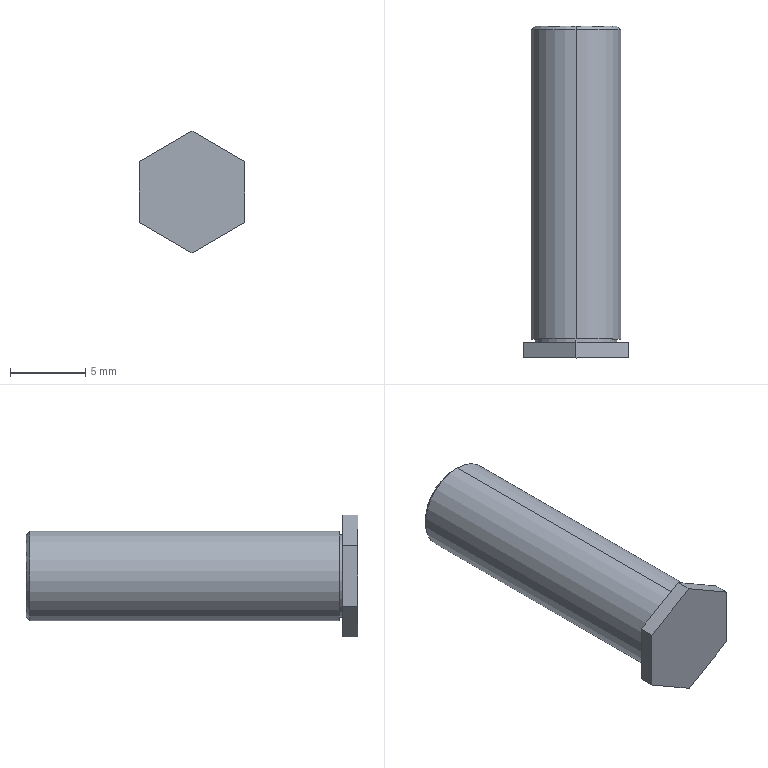Part | NX | features BREP 1 | 1 solid | 21 faces | box 7 x 22 x 8.083 mm | volume 461.807 mm3 | plane 11 | cylinder 6 | cone 4 | commonest cylinder face diameters 3.3 x2 5.45 x2 5.95 x2
STEP:
#1=CARTESIAN_POINT('',(300.5,43.15,424.025));
#2=VERTEX_POINT('',#1);
#3=CARTESIAN_POINT('',(300.5,43.15,429.975));
#4=VERTEX_POINT('',#3);
#5=CARTESIAN_POINT('',(300.5,43.15,427.));
#6=DIRECTION('',(0.,-1.,0.));
#7=DIRECTION('',(0.,0.,-1.));
#8=AXIS2_PLACEMENT_3D('',#5,#6,#7);
#9=CIRCLE('',#8,2.975);
#10=EDGE_CURVE('',#2,#4,#9,.T.);
#11=ORIENTED_EDGE('',*,*,#10,.T.);
#12=CARTESIAN_POINT('',(300.5,22.65,429.975));
#13=VERTEX_POINT('',#12);
#14=CARTESIAN_POINT('',(300.5,31.4,429.975));
#15=DIRECTION('',(0.,-1.,0.));
#16=VECTOR('',#15,1000.);
#17=LINE('',#14,#16);
#18=EDGE_CURVE('',#13,#4,#17,.F.);
#19=ORIENTED_EDGE('',*,*,#18,.F.);
#20=CARTESIAN_POINT('',(300.5,22.65,424.025));
#21=VERTEX_POINT('',#20);
#22=CARTESIAN_POINT('',(300.5,22.65,427.));
#23=DIRECTION('',(0.,1.,0.));
#24=DIRECTION('',(0.,0.,-1.));
#25=AXIS2_PLACEMENT_3D('',#22,#23,#24);
#26=CIRCLE('',#25,2.975);
#27=EDGE_CURVE('',#13,#21,#26,.T.);
#28=ORIENTED_EDGE('',*,*,#27,.T.);
#29=CARTESIAN_POINT('',(300.5,31.4,424.025));
#30=DIRECTION('',(0.,-1.,0.));
#31=VECTOR('',#30,1000.);
#32=LINE('',#29,#31);
#33=EDGE_CURVE('',#21,#2,#32,.F.);
#34=ORIENTED_EDGE('',*,*,#33,.T.);
#35=EDGE_LOOP('',(#11,#19,#28,#34));
#36=FACE_BOUND('',#35,.T.);
#37=CARTESIAN_POINT('',(300.5,31.4,427.));
#38=DIRECTION('',(0.,-1.,0.));
#39=DIRECTION('',(0.,0.,1.));
#40=AXIS2_PLACEMENT_3D('',#37,#38,#39);
#41=CYLINDRICAL_SURFACE('',#40,2.975);
#42=ADVANCED_FACE('',(#36),#41,.T.);
#43=CARTESIAN_POINT('',(300.5,43.4,424.275));
#44=VERTEX_POINT('',#43);
#45=CARTESIAN_POINT('',(300.5,43.4,429.725));
#46=VERTEX_POINT('',#45);
#47=CARTESIAN_POINT('',(300.5,43.4,427.));
#48=DIRECTION('',(0.,-1.,0.));
#49=DIRECTION('',(0.,0.,-1.));
#50=AXIS2_PLACEMENT_3D('',#47,#48,#49);
#51=CIRCLE('',#50,2.725);
#52=EDGE_CURVE('',#44,#46,#51,.T.);
#53=ORIENTED_EDGE('',*,*,#52,.T.);
#54=CARTESIAN_POINT('',(300.5,43.15,429.975));
#55=DIRECTION('',(0.,-0.7071,0.7071));
#56=VECTOR('',#55,1000.);
#57=LINE('',#54,#56);
#58=EDGE_CURVE('',#4,#46,#57,.F.);
#59=ORIENTED_EDGE('',*,*,#58,.F.);
#60=ORIENTED_EDGE('',*,*,#10,.F.);
#61=CARTESIAN_POINT('',(300.5,43.15,424.025));
#62=DIRECTION('',(0.,-0.7071,-0.7071));
#63=VECTOR('',#62,1000.);
#64=LINE('',#61,#63);
#65=EDGE_CURVE('',#2,#44,#64,.F.);
#66=ORIENTED_EDGE('',*,*,#65,.T.);
#67=EDGE_LOOP('',(#53,#59,#60,#66));
#68=FACE_BOUND('',#67,.T.);
#69=CARTESIAN_POINT('',(300.5,43.15,427.));
#70=DIRECTION('',(0.,-1.,0.));
#71=DIRECTION('',(0.,0.,1.));
#72=AXIS2_PLACEMENT_3D('',#69,#70,#71);
#73=CONICAL_SURFACE('',#72,2.975,0.7854);
#74=ADVANCED_FACE('',(#68),#73,.T.);
#75=CARTESIAN_POINT('',(300.5,22.4,429.725));
#76=VERTEX_POINT('',#75);
#77=CARTESIAN_POINT('',(300.5,22.4,424.275));
#78=VERTEX_POINT('',#77);
#79=CARTESIAN_POINT('',(300.5,22.4,427.));
#80=DIRECTION('',(0.,1.,0.));
#81=DIRECTION('',(0.,0.,1.));
#82=AXIS2_PLACEMENT_3D('',#79,#80,#81);
#83=CIRCLE('',#82,2.725);
#84=EDGE_CURVE('',#76,#78,#83,.T.);
#85=ORIENTED_EDGE('',*,*,#84,.T.);
#86=CARTESIAN_POINT('',(300.5,22.65,424.275));
#87=VERTEX_POINT('',#86);
#88=CARTESIAN_POINT('',(300.5,-1.133,424.275));
#89=DIRECTION('',(0.,1.,0.));
#90=VECTOR('',#89,1000.);
#91=LINE('',#88,#90);
#92=EDGE_CURVE('',#78,#87,#91,.T.);
#93=ORIENTED_EDGE('',*,*,#92,.T.);
#94=CARTESIAN_POINT('',(300.5,22.65,429.725));
#95=VERTEX_POINT('',#94);
#96=CARTESIAN_POINT('',(300.5,22.65,427.));
#97=DIRECTION('',(0.,-1.,0.));
#98=DIRECTION('',(0.,0.,1.));
#99=AXIS2_PLACEMENT_3D('',#96,#97,#98);
#100=CIRCLE('',#99,2.725);
#101=EDGE_CURVE('',#87,#95,#100,.T.);
#102=ORIENTED_EDGE('',*,*,#101,.T.);
#103=CARTESIAN_POINT('',(300.5,-1.133,429.725));
#104=DIRECTION('',(0.,1.,0.));
#105=VECTOR('',#104,1000.);
#106=LINE('',#103,#105);
#107=EDGE_CURVE('',#76,#95,#106,.T.);
#108=ORIENTED_EDGE('',*,*,#107,.F.);
#109=EDGE_LOOP('',(#85,#93,#102,#108));
#110=FACE_BOUND('',#109,.T.);
#111=CARTESIAN_POINT('',(300.5,-1.133,427.));
#112=DIRECTION('',(0.,1.,0.));
#113=DIRECTION('',(0.,0.,-1.));
#114=AXIS2_PLACEMENT_3D('',#111,#112,#113);
#115=CYLINDRICAL_SURFACE('',#114,2.725);
#116=ADVANCED_FACE('',(#110),#115,.T.);
#117=CARTESIAN_POINT('',(300.5,43.15,425.35));
#118=VERTEX_POINT('',#117);
#119=CARTESIAN_POINT('',(300.5,43.15,428.65));
#120=VERTEX_POINT('',#119);
#121=CARTESIAN_POINT('',(300.5,43.15,427.));
#122=DIRECTION('',(0.,1.,0.));
#123=DIRECTION('',(0.,0.,1.));
#124=AXIS2_PLACEMENT_3D('',#121,#122,#123);
#125=CIRCLE('',#124,1.65);
#126=EDGE_CURVE('',#118,#120,#125,.T.);
#127=ORIENTED_EDGE('',*,*,#126,.F.);
#128=CARTESIAN_POINT('',(300.5,43.4,425.1));
#129=VERTEX_POINT('',#128);
#130=CARTESIAN_POINT('',(300.5,43.4,425.1));
#131=DIRECTION('',(0.,0.7071,-0.7071));
#132=VECTOR('',#131,1000.);
#133=LINE('',#130,#132);
#134=EDGE_CURVE('',#118,#129,#133,.T.);
#135=ORIENTED_EDGE('',*,*,#134,.T.);
#136=CARTESIAN_POINT('',(300.5,43.4,428.9));
#137=VERTEX_POINT('',#136);
#138=CARTESIAN_POINT('',(300.5,43.4,427.));
#139=DIRECTION('',(0.,-1.,0.));
#140=DIRECTION('',(0.,0.,1.));
#141=AXIS2_PLACEMENT_3D('',#138,#139,#140);
#142=CIRCLE('',#141,1.9);
#143=EDGE_CURVE('',#137,#129,#142,.T.);
#144=ORIENTED_EDGE('',*,*,#143,.F.);
#145=CARTESIAN_POINT('',(300.5,43.4,428.9));
#146=DIRECTION('',(0.,0.7071,0.7071));
#147=VECTOR('',#146,1000.);
#148=LINE('',#145,#147);
#149=EDGE_CURVE('',#120,#137,#148,.T.);
#150=ORIENTED_EDGE('',*,*,#149,.F.);
#151=EDGE_LOOP('',(#127,#135,#144,#150));
#152=FACE_BOUND('',#151,.T.);
#153=CARTESIAN_POINT('',(300.5,43.4,427.));
#154=DIRECTION('',(0.,1.,0.));
#155=DIRECTION('',(0.,0.,-1.));
#156=AXIS2_PLACEMENT_3D('',#153,#154,#155);
#157=CONICAL_SURFACE('',#156,1.9,0.7854);
#158=ADVANCED_FACE('',(#152),#157,.F.);
#159=CARTESIAN_POINT('',(300.5,24.4,425.35));
#160=VERTEX_POINT('',#159);
#161=CARTESIAN_POINT('',(300.5,24.4,428.65));
#162=VERTEX_POINT('',#161);
#163=CARTESIAN_POINT('',(300.5,24.4,427.));
#164=DIRECTION('',(0.,1.,0.));
#165=DIRECTION('',(0.,0.,1.));
#166=AXIS2_PLACEMENT_3D('',#163,#164,#165);
#167=CIRCLE('',#166,1.65);
#168=EDGE_CURVE('',#160,#162,#167,.T.);
#169=ORIENTED_EDGE('',*,*,#168,.F.);
#170=CARTESIAN_POINT('',(300.5,24.4,425.35));
#171=DIRECTION('',(0.,1.,0.));
#172=VECTOR('',#171,1000.);
#173=LINE('',#170,#172);
#174=EDGE_CURVE('',#160,#118,#173,.T.);
#175=ORIENTED_EDGE('',*,*,#174,.T.);
#176=ORIENTED_EDGE('',*,*,#126,.T.);
#177=CARTESIAN_POINT('',(300.5,24.4,428.65));
#178=DIRECTION('',(0.,1.,0.));
#179=VECTOR('',#178,1000.);
#180=LINE('',#177,#179);
#181=EDGE_CURVE('',#162,#120,#180,.T.);
#182=ORIENTED_EDGE('',*,*,#181,.F.);
#183=EDGE_LOOP('',(#169,#175,#176,#182));
#184=FACE_BOUND('',#183,.T.);
#185=CARTESIAN_POINT('',(300.5,24.4,427.));
#186=DIRECTION('',(0.,1.,0.));
#187=DIRECTION('',(0.,0.,-1.));
#188=AXIS2_PLACEMENT_3D('',#185,#186,#187);
#189=CYLINDRICAL_SURFACE('',#188,1.65);
#190=ADVANCED_FACE('',(#184),#189,.F.);
#191=ORIENTED_EDGE('',*,*,#18,.T.);
#192=CARTESIAN_POINT('',(300.5,43.15,427.));
#193=DIRECTION('',(0.,-1.,0.));
#194=DIRECTION('',(0.,0.,-1.));
#195=AXIS2_PLACEMENT_3D('',#192,#193,#194);
#196=CIRCLE('',#195,2.975);
#197=EDGE_CURVE('',#4,#2,#196,.T.);
#198=ORIENTED_EDGE('',*,*,#197,.T.);
#199=ORIENTED_EDGE('',*,*,#33,.F.);
#200=CARTESIAN_POINT('',(300.5,22.65,427.));
#201=DIRECTION('',(0.,1.,0.));
#202=DIRECTION('',(0.,0.,-1.));
#203=AXIS2_PLACEMENT_3D('',#200,#201,#202);
#204=CIRCLE('',#203,2.975);
#205=EDGE_CURVE('',#21,#13,#204,.T.);
#206=ORIENTED_EDGE('',*,*,#205,.T.);
#207=EDGE_LOOP('',(#191,#198,#199,#206));
#208=FACE_BOUND('',#207,.T.);
#209=CARTESIAN_POINT('',(300.5,31.4,427.));
#210=DIRECTION('',(0.,-1.,0.));
#211=DIRECTION('',(0.,0.,1.));
#212=AXIS2_PLACEMENT_3D('',#209,#210,#211);
#213=CYLINDRICAL_SURFACE('',#212,2.975);
#214=ADVANCED_FACE('',(#208),#213,.T.);
#215=ORIENTED_EDGE('',*,*,#205,.F.);
#216=ORIENTED_EDGE('',*,*,#27,.F.);
#217=EDGE_LOOP('',(#215,#216));
#218=FACE_BOUND('',#217,.T.);
#219=CARTESIAN_POINT('',(300.5,22.65,427.));
#220=DIRECTION('',(0.,-1.,0.));
#221=DIRECTION('',(0.,0.,1.));
#222=AXIS2_PLACEMENT_3D('',#219,#220,#221);
#223=CIRCLE('',#222,2.725);
#224=EDGE_CURVE('',#95,#87,#223,.T.);
#225=ORIENTED_EDGE('',*,*,#224,.F.);
#226=ORIENTED_EDGE('',*,*,#101,.F.);
#227=EDGE_LOOP('',(#225,#226));
#228=FACE_BOUND('',#227,.T.);
#229=CARTESIAN_POINT('',(300.5,22.65,427.));
#230=DIRECTION('',(0.,1.,0.));
#231=DIRECTION('',(0.,0.,-1.));
#232=AXIS2_PLACEMENT_3D('',#229,#230,#231);
#233=PLANE('',#232);
#234=ADVANCED_FACE('',(#218,#228),#233,.F.);
#235=ORIENTED_EDGE('',*,*,#58,.T.);
#236=CARTESIAN_POINT('',(300.5,43.4,427.));
#237=DIRECTION('',(0.,-1.,0.));
#238=DIRECTION('',(0.,0.,-1.));
#239=AXIS2_PLACEMENT_3D('',#236,#237,#238);
#240=CIRCLE('',#239,2.725);
#241=EDGE_CURVE('',#46,#44,#240,.T.);
#242=ORIENTED_EDGE('',*,*,#241,.T.);
#243=ORIENTED_EDGE('',*,*,#65,.F.);
#244=ORIENTED_EDGE('',*,*,#197,.F.);
#245=EDGE_LOOP('',(#235,#242,#243,#244));
#246=FACE_BOUND('',#245,.T.);
#247=CARTESIAN_POINT('',(300.5,43.15,427.));
#248=DIRECTION('',(0.,-1.,0.));
#249=DIRECTION('',(0.,0.,1.));
#250=AXIS2_PLACEMENT_3D('',#247,#248,#249);
#251=CONICAL_SURFACE('',#250,2.975,0.7854);
#252=ADVANCED_FACE('',(#246),#251,.T.);
#253=ORIENTED_EDGE('',*,*,#92,.F.);
#254=CARTESIAN_POINT('',(300.5,22.4,427.));
#255=DIRECTION('',(0.,1.,0.));
#256=DIRECTION('',(0.,0.,1.));
#257=AXIS2_PLACEMENT_3D('',#254,#255,#256);
#258=CIRCLE('',#257,2.725);
#259=EDGE_CURVE('',#78,#76,#258,.T.);
#260=ORIENTED_EDGE('',*,*,#259,.T.);
#261=ORIENTED_EDGE('',*,*,#107,.T.);
#262=ORIENTED_EDGE('',*,*,#224,.T.);
#263=EDGE_LOOP('',(#253,#260,#261,#262));
#264=FACE_BOUND('',#263,.T.);
#265=CARTESIAN_POINT('',(300.5,-1.133,427.));
#266=DIRECTION('',(0.,1.,0.));
#267=DIRECTION('',(0.,0.,-1.));
#268=AXIS2_PLACEMENT_3D('',#265,#266,#267);
#269=CYLINDRICAL_SURFACE('',#268,2.725);
#270=ADVANCED_FACE('',(#264),#269,.T.);
#271=ORIENTED_EDGE('',*,*,#52,.F.);
#272=ORIENTED_EDGE('',*,*,#241,.F.);
#273=EDGE_LOOP('',(#271,#272));
#274=FACE_BOUND('',#273,.T.);
#275=ORIENTED_EDGE('',*,*,#143,.T.);
#276=CARTESIAN_POINT('',(300.5,43.4,427.));
#277=DIRECTION('',(0.,-1.,0.));
#278=DIRECTION('',(0.,0.,1.));
#279=AXIS2_PLACEMENT_3D('',#276,#277,#278);
#280=CIRCLE('',#279,1.9);
#281=EDGE_CURVE('',#129,#137,#280,.T.);
#282=ORIENTED_EDGE('',*,*,#281,.T.);
#283=EDGE_LOOP('',(#275,#282));
#284=FACE_BOUND('',#283,.T.);
#285=CARTESIAN_POINT('',(300.5,43.4,427.));
#286=DIRECTION('',(0.,1.,0.));
#287=DIRECTION('',(0.,0.,-1.));
#288=AXIS2_PLACEMENT_3D('',#285,#286,#287);
#289=PLANE('',#288);
#290=ADVANCED_FACE('',(#274,#284),#289,.T.);
#291=CARTESIAN_POINT('',(300.5,22.4,422.959));
#292=VERTEX_POINT('',#291);
#293=CARTESIAN_POINT('',(297.,22.4,424.979));
#294=VERTEX_POINT('',#293);
#295=CARTESIAN_POINT('',(300.5,22.4,422.959));
#296=DIRECTION('',(-0.866,0.,0.5));
#297=VECTOR('',#296,1000.);
#298=LINE('',#295,#297);
#299=EDGE_CURVE('',#292,#294,#298,.T.);
#300=ORIENTED_EDGE('',*,*,#299,.T.);
#301=CARTESIAN_POINT('',(297.,22.4,429.021));
#302=VERTEX_POINT('',#301);
#303=CARTESIAN_POINT('',(297.,22.4,427.));
#304=DIRECTION('',(0.,0.,1.));
#305=VECTOR('',#304,1000.);
#306=LINE('',#303,#305);
#307=EDGE_CURVE('',#294,#302,#306,.T.);
#308=ORIENTED_EDGE('',*,*,#307,.T.);
#309=CARTESIAN_POINT('',(300.5,22.4,431.041));
#310=VERTEX_POINT('',#309);
#311=CARTESIAN_POINT('',(297.,22.4,429.021));
#312=DIRECTION('',(0.866,0.,0.5));
#313=VECTOR('',#312,1000.);
#314=LINE('',#311,#313);
#315=EDGE_CURVE('',#302,#310,#314,.T.);
#316=ORIENTED_EDGE('',*,*,#315,.T.);
#317=CARTESIAN_POINT('',(304.,22.4,429.021));
#318=VERTEX_POINT('',#317);
#319=CARTESIAN_POINT('',(300.5,22.4,431.041));
#320=DIRECTION('',(0.866,0.,-0.5));
#321=VECTOR('',#320,1000.);
#322=LINE('',#319,#321);
#323=EDGE_CURVE('',#310,#318,#322,.T.);
#324=ORIENTED_EDGE('',*,*,#323,.T.);
#325=CARTESIAN_POINT('',(304.,22.4,424.979));
#326=VERTEX_POINT('',#325);
#327=CARTESIAN_POINT('',(304.,22.4,427.));
#328=DIRECTION('',(0.,0.,-1.));
#329=VECTOR('',#328,1000.);
#330=LINE('',#327,#329);
#331=EDGE_CURVE('',#318,#326,#330,.T.);
#332=ORIENTED_EDGE('',*,*,#331,.T.);
#333=CARTESIAN_POINT('',(304.,22.4,424.979));
#334=DIRECTION('',(-0.866,0.,-0.5));
#335=VECTOR('',#334,1000.);
#336=LINE('',#333,#335);
#337=EDGE_CURVE('',#326,#292,#336,.T.);
#338=ORIENTED_EDGE('',*,*,#337,.T.);
#339=EDGE_LOOP('',(#300,#308,#316,#324,#332,#338));
#340=FACE_BOUND('',#339,.T.);
#341=ORIENTED_EDGE('',*,*,#84,.F.);
#342=ORIENTED_EDGE('',*,*,#259,.F.);
#343=EDGE_LOOP('',(#341,#342));
#344=FACE_BOUND('',#343,.T.);
#345=CARTESIAN_POINT('',(300.5,22.4,427.));
#346=DIRECTION('',(0.,1.,0.));
#347=DIRECTION('',(0.,0.,-1.));
#348=AXIS2_PLACEMENT_3D('',#345,#346,#347);
#349=PLANE('',#348);
#350=ADVANCED_FACE('',(#340,#344),#349,.T.);
#351=ORIENTED_EDGE('',*,*,#134,.F.);
#352=CARTESIAN_POINT('',(300.5,43.15,427.));
#353=DIRECTION('',(0.,1.,0.));
#354=DIRECTION('',(0.,0.,1.));
#355=AXIS2_PLACEMENT_3D('',#352,#353,#354);
#356=CIRCLE('',#355,1.65);
#357=EDGE_CURVE('',#120,#118,#356,.T.);
#358=ORIENTED_EDGE('',*,*,#357,.F.);
#359=ORIENTED_EDGE('',*,*,#149,.T.);
#360=ORIENTED_EDGE('',*,*,#281,.F.);
#361=EDGE_LOOP('',(#351,#358,#359,#360));
#362=FACE_BOUND('',#361,.T.);
#363=CARTESIAN_POINT('',(300.5,43.4,427.));
#364=DIRECTION('',(0.,1.,0.));
#365=DIRECTION('',(0.,0.,-1.));
#366=AXIS2_PLACEMENT_3D('',#363,#364,#365);
#367=CONICAL_SURFACE('',#366,1.9,0.7854);
#368=ADVANCED_FACE('',(#362),#367,.F.);
#369=CARTESIAN_POINT('',(297.,21.4,424.979));
#370=VERTEX_POINT('',#369);
#371=CARTESIAN_POINT('',(297.,22.4,424.979));
#372=DIRECTION('',(0.,1.,0.));
#373=VECTOR('',#372,1000.);
#374=LINE('',#371,#373);
#375=EDGE_CURVE('',#370,#294,#374,.T.);
#376=ORIENTED_EDGE('',*,*,#375,.F.);
#377=CARTESIAN_POINT('',(297.,21.4,429.021));
#378=VERTEX_POINT('',#377);
#379=CARTESIAN_POINT('',(297.,21.4,424.979));
#380=DIRECTION('',(0.,0.,-1.));
#381=VECTOR('',#380,1000.);
#382=LINE('',#379,#381);
#383=EDGE_CURVE('',#378,#370,#382,.T.);
#384=ORIENTED_EDGE('',*,*,#383,.F.);
#385=CARTESIAN_POINT('',(297.,22.4,429.021));
#386=DIRECTION('',(0.,-1.,0.));
#387=VECTOR('',#386,1000.);
#388=LINE('',#385,#387);
#389=EDGE_CURVE('',#302,#378,#388,.T.);
#390=ORIENTED_EDGE('',*,*,#389,.F.);
#391=ORIENTED_EDGE('',*,*,#307,.F.);
#392=EDGE_LOOP('',(#376,#384,#390,#391));
#393=FACE_BOUND('',#392,.T.);
#394=CARTESIAN_POINT('',(297.,22.4,424.979));
#395=DIRECTION('',(1.,0.,0.));
#396=DIRECTION('',(0.,0.,1.));
#397=AXIS2_PLACEMENT_3D('',#394,#395,#396);
#398=PLANE('',#397);
#399=ADVANCED_FACE('',(#393),#398,.F.);
#400=CARTESIAN_POINT('',(300.5,21.4,422.959));
#401=VERTEX_POINT('',#400);
#402=CARTESIAN_POINT('',(300.5,22.4,422.959));
#403=DIRECTION('',(0.,1.,0.));
#404=VECTOR('',#403,1000.);
#405=LINE('',#402,#404);
#406=EDGE_CURVE('',#401,#292,#405,.T.);
#407=ORIENTED_EDGE('',*,*,#406,.F.);
#408=CARTESIAN_POINT('',(300.5,21.4,422.959));
#409=DIRECTION('',(0.866,0.,-0.5));
#410=VECTOR('',#409,1000.);
#411=LINE('',#408,#410);
#412=EDGE_CURVE('',#370,#401,#411,.T.);
#413=ORIENTED_EDGE('',*,*,#412,.F.);
#414=ORIENTED_EDGE('',*,*,#375,.T.);
#415=ORIENTED_EDGE('',*,*,#299,.F.);
#416=EDGE_LOOP('',(#407,#413,#414,#415));
#417=FACE_BOUND('',#416,.T.);
#418=CARTESIAN_POINT('',(300.5,22.4,422.959));
#419=DIRECTION('',(0.5,0.,0.866));
#420=DIRECTION('',(-0.866,0.,0.5));
#421=AXIS2_PLACEMENT_3D('',#418,#419,#420);
#422=PLANE('',#421);
#423=ADVANCED_FACE('',(#417),#422,.F.);
#424=CARTESIAN_POINT('',(304.,21.4,424.979));
#425=VERTEX_POINT('',#424);
#426=CARTESIAN_POINT('',(304.,22.4,424.979));
#427=DIRECTION('',(0.,1.,0.));
#428=VECTOR('',#427,1000.);
#429=LINE('',#426,#428);
#430=EDGE_CURVE('',#425,#326,#429,.T.);
#431=ORIENTED_EDGE('',*,*,#430,.F.);
#432=CARTESIAN_POINT('',(304.,21.4,424.979));
#433=DIRECTION('',(0.866,0.,0.5));
#434=VECTOR('',#433,1000.);
#435=LINE('',#432,#434);
#436=EDGE_CURVE('',#401,#425,#435,.T.);
#437=ORIENTED_EDGE('',*,*,#436,.F.);
#438=ORIENTED_EDGE('',*,*,#406,.T.);
#439=ORIENTED_EDGE('',*,*,#337,.F.);
#440=EDGE_LOOP('',(#431,#437,#438,#439));
#441=FACE_BOUND('',#440,.T.);
#442=CARTESIAN_POINT('',(304.,22.4,424.979));
#443=DIRECTION('',(-0.5,0.,0.866));
#444=DIRECTION('',(-0.866,0.,-0.5));
#445=AXIS2_PLACEMENT_3D('',#442,#443,#444);
#446=PLANE('',#445);
#447=ADVANCED_FACE('',(#441),#446,.F.);
#448=CARTESIAN_POINT('',(304.,21.4,429.021));
#449=VERTEX_POINT('',#448);
#450=CARTESIAN_POINT('',(304.,22.4,429.021));
#451=DIRECTION('',(0.,1.,0.));
#452=VECTOR('',#451,1000.);
#453=LINE('',#450,#452);
#454=EDGE_CURVE('',#449,#318,#453,.T.);
#455=ORIENTED_EDGE('',*,*,#454,.F.);
#456=CARTESIAN_POINT('',(304.,21.4,429.021));
#457=DIRECTION('',(0.,0.,1.));
#458=VECTOR('',#457,1000.);
#459=LINE('',#456,#458);
#460=EDGE_CURVE('',#425,#449,#459,.T.);
#461=ORIENTED_EDGE('',*,*,#460,.F.);
#462=ORIENTED_EDGE('',*,*,#430,.T.);
#463=ORIENTED_EDGE('',*,*,#331,.F.);
#464=EDGE_LOOP('',(#455,#461,#462,#463));
#465=FACE_BOUND('',#464,.T.);
#466=CARTESIAN_POINT('',(304.,22.4,429.021));
#467=DIRECTION('',(-1.,0.,0.));
#468=DIRECTION('',(0.,0.,-1.));
#469=AXIS2_PLACEMENT_3D('',#466,#467,#468);
#470=PLANE('',#469);
#471=ADVANCED_FACE('',(#465),#470,.F.);
#472=CARTESIAN_POINT('',(300.5,21.4,431.041));
#473=VERTEX_POINT('',#472);
#474=CARTESIAN_POINT('',(300.5,22.4,431.041));
#475=DIRECTION('',(0.,1.,0.));
#476=VECTOR('',#475,1000.);
#477=LINE('',#474,#476);
#478=EDGE_CURVE('',#473,#310,#477,.T.);
#479=ORIENTED_EDGE('',*,*,#478,.F.);
#480=CARTESIAN_POINT('',(300.5,21.4,431.041));
#481=DIRECTION('',(-0.866,0.,0.5));
#482=VECTOR('',#481,1000.);
#483=LINE('',#480,#482);
#484=EDGE_CURVE('',#449,#473,#483,.T.);
#485=ORIENTED_EDGE('',*,*,#484,.F.);
#486=ORIENTED_EDGE('',*,*,#454,.T.);
#487=ORIENTED_EDGE('',*,*,#323,.F.);
#488=EDGE_LOOP('',(#479,#485,#486,#487));
#489=FACE_BOUND('',#488,.T.);
#490=CARTESIAN_POINT('',(300.5,22.4,431.041));
#491=DIRECTION('',(-0.5,0.,-0.866));
#492=DIRECTION('',(0.866,0.,-0.5));
#493=AXIS2_PLACEMENT_3D('',#490,#491,#492);
#494=PLANE('',#493);
#495=ADVANCED_FACE('',(#489),#494,.F.);
#496=ORIENTED_EDGE('',*,*,#389,.T.);
#497=CARTESIAN_POINT('',(297.,21.4,429.021));
#498=DIRECTION('',(-0.866,0.,-0.5));
#499=VECTOR('',#498,1000.);
#500=LINE('',#497,#499);
#501=EDGE_CURVE('',#473,#378,#500,.T.);
#502=ORIENTED_EDGE('',*,*,#501,.F.);
#503=ORIENTED_EDGE('',*,*,#478,.T.);
#504=ORIENTED_EDGE('',*,*,#315,.F.);
#505=EDGE_LOOP('',(#496,#502,#503,#504));
#506=FACE_BOUND('',#505,.T.);
#507=CARTESIAN_POINT('',(297.,22.4,429.021));
#508=DIRECTION('',(0.5,0.,-0.866));
#509=DIRECTION('',(0.866,0.,0.5));
#510=AXIS2_PLACEMENT_3D('',#507,#508,#509);
#511=PLANE('',#510);
#512=ADVANCED_FACE('',(#506),#511,.F.);
#513=ORIENTED_EDGE('',*,*,#174,.F.);
#514=CARTESIAN_POINT('',(300.5,24.4,427.));
#515=DIRECTION('',(0.,1.,0.));
#516=DIRECTION('',(0.,0.,1.));
#517=AXIS2_PLACEMENT_3D('',#514,#515,#516);
#518=CIRCLE('',#517,1.65);
#519=EDGE_CURVE('',#162,#160,#518,.T.);
#520=ORIENTED_EDGE('',*,*,#519,.F.);
#521=ORIENTED_EDGE('',*,*,#181,.T.);
#522=ORIENTED_EDGE('',*,*,#357,.T.);
#523=EDGE_LOOP('',(#513,#520,#521,#522));
#524=FACE_BOUND('',#523,.T.);
#525=CARTESIAN_POINT('',(300.5,24.4,427.));
#526=DIRECTION('',(0.,1.,0.));
#527=DIRECTION('',(0.,0.,-1.));
#528=AXIS2_PLACEMENT_3D('',#525,#526,#527);
#529=CYLINDRICAL_SURFACE('',#528,1.65);
#530=ADVANCED_FACE('',(#524),#529,.F.);
#531=ORIENTED_EDGE('',*,*,#460,.T.);
#532=ORIENTED_EDGE('',*,*,#484,.T.);
#533=ORIENTED_EDGE('',*,*,#501,.T.);
#534=ORIENTED_EDGE('',*,*,#383,.T.);
#535=ORIENTED_EDGE('',*,*,#412,.T.);
#536=ORIENTED_EDGE('',*,*,#436,.T.);
#537=EDGE_LOOP('',(#531,#532,#533,#534,#535,#536));
#538=FACE_BOUND('',#537,.T.);
#539=CARTESIAN_POINT('',(300.5,21.4,427.));
#540=DIRECTION('',(0.,1.,0.));
#541=DIRECTION('',(0.,0.,-1.));
#542=AXIS2_PLACEMENT_3D('',#539,#540,#541);
#543=PLANE('',#542);
#544=ADVANCED_FACE('',(#538),#543,.F.);
#545=ORIENTED_EDGE('',*,*,#519,.T.);
#546=ORIENTED_EDGE('',*,*,#168,.T.);
#547=EDGE_LOOP('',(#545,#546));
#548=FACE_BOUND('',#547,.T.);
#549=CARTESIAN_POINT('',(300.5,24.4,427.));
#550=DIRECTION('',(0.,1.,0.));
#551=DIRECTION('',(0.,0.,-1.));
#552=AXIS2_PLACEMENT_3D('',#549,#550,#551);
#553=PLANE('',#552);
#554=ADVANCED_FACE('',(#548),#553,.T.);
#555=CLOSED_SHELL('',(#42,#74,#116,#158,#190,#214,#234,#252,#270,#290,#350,#368,#399,#423,#447,#471,#495,#512,#530,#544,#554));
#556=MANIFOLD_SOLID_BREP('',#555);
#557=(LENGTH_UNIT()NAMED_UNIT(*)SI_UNIT(.MILLI.,.METRE.));
#558=UNCERTAINTY_MEASURE_WITH_UNIT(LENGTH_MEASURE(0.00001),#557,'','');
#559=(NAMED_UNIT(*)PLANE_ANGLE_UNIT()SI_UNIT($,.RADIAN.));
#560=(NAMED_UNIT(*)SI_UNIT($,.STERADIAN.)SOLID_ANGLE_UNIT());
#561=(GEOMETRIC_REPRESENTATION_CONTEXT(3)GLOBAL_UNCERTAINTY_ASSIGNED_CONTEXT((#558))GLOBAL_UNIT_ASSIGNED_CONTEXT((#557,#559,#560))REPRESENTATION_CONTEXT('',''));
#562=ADVANCED_BREP_SHAPE_REPRESENTATION('',(#556),#561);